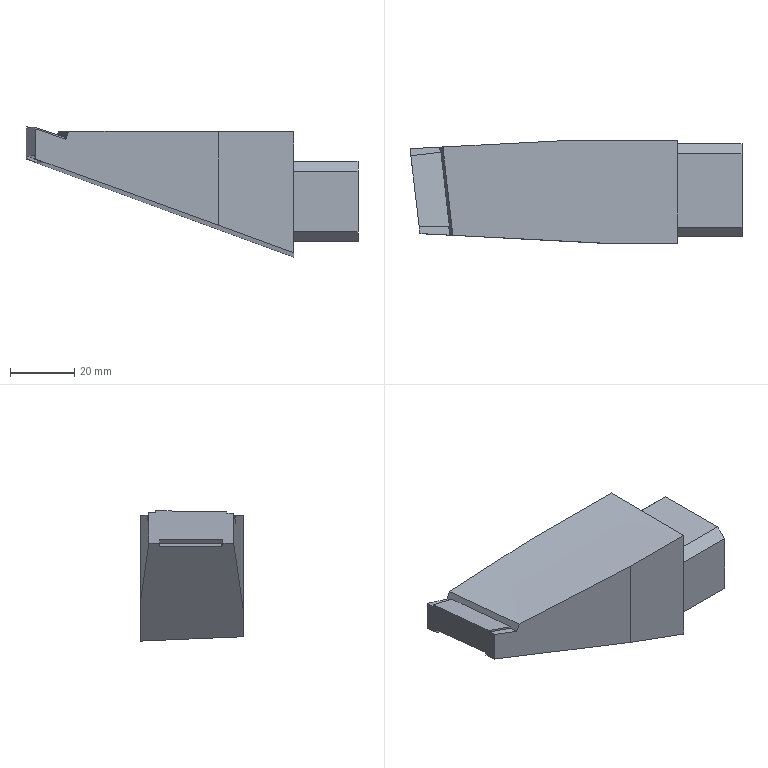Part | STEP file | P011002S002-002 | 1 solid | 61 faces | box 103.644 x 32 x 40.64 mm | volume 72911 mm3 | plane 35 | other 11 | cone 7 | spline 5 | cylinder 3 | commonest cylinder face diameters 6.8 x1 7.973 x1 8 x1